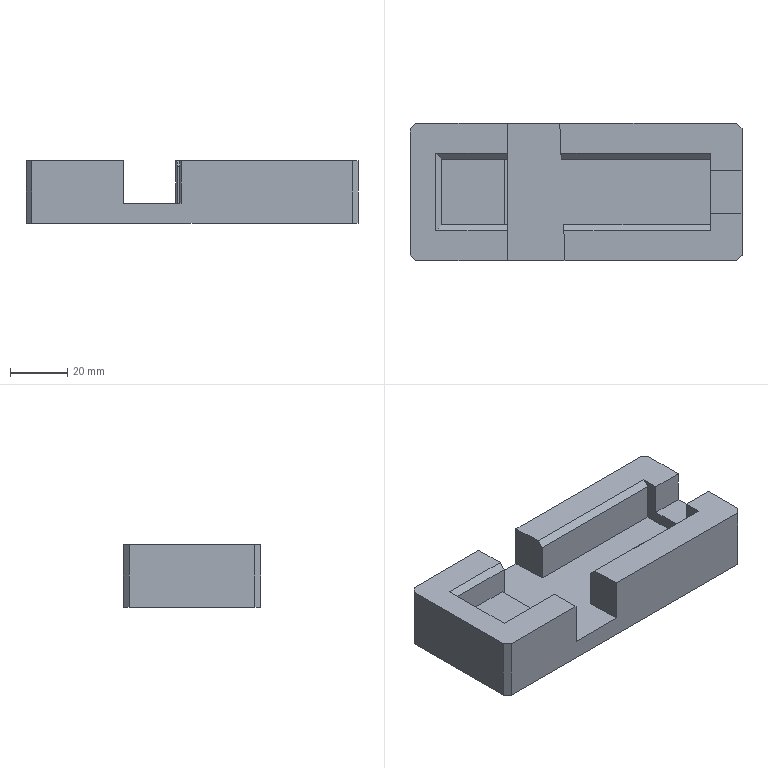Part | STEP file | PN_0002 | 1 solid | 38 faces | box 116 x 48 x 22 mm | volume 82271 mm3 | plane 34 | cylinder 4 | commonest cylinder face diameters 6 x4